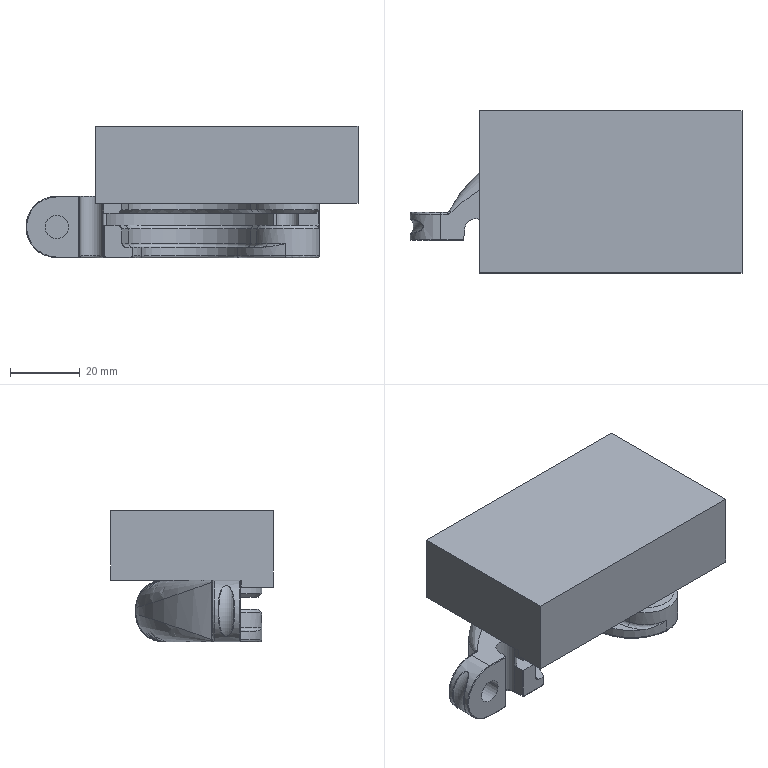NC program | NX | posted with a generic post | part box 94.951 x 46.35 x 37.6 mm
Lines 1740 to 2347 of 15115:
(ZLEVEL_PROFILE_COPY , TOOL : D6R0.5)
N3418 T23 M6
N3420 G54
N3422 G17 G0 G90 X42.811 Y-3.515 S6500 M3
N3424 G43 Z20. H23
N3426 Z-0.004
N3428 G94 G3 X42.99 Y-4.167 R2. F2500.
N3430 G2 X21.925 Y-11.674 R-11.232
N3432 G1 X20.25 Y-5.033
N3434 G3 X-10.601 Y-5.035 R15.909
N3436 G1 X-12.275 Y-11.674
N3438 G2 X-12.624 Y-12.804 R11.241
N3440 G3 X-12.738 Y-13.311 R2.
N3442 G1 X-12.683 Y-13.314 Z-0.011 F8000.
N3444 G2 X-12.57 Y-12.81 R2. F2500.
N3446 G3 X-12.223 Y-11.687 R11.295
N3448 G1 X-10.549 Y-5.048
N3450 G2 X20.199 Y-5.048 R15.855
N3452 G1 X21.873 Y-11.687
N3454 G3 X43.054 Y-4.145 R-11.292
N3456 G2 X42.876 Y-3.495 R2.
N3458 G1 X43.042 Y-3.715 Z-0.019 F8000.
N3460 G3 X43.106 Y-4.136 R1. F2500.
N3462 G2 X21.824 Y-11.699 R-11.343
N3464 G1 X20.15 Y-5.06
N3466 G3 X-10.499 Y-5.06 R15.804
N3468 G1 X-12.174 Y-11.699
N3470 G2 X-12.518 Y-12.817 R11.346
N3472 G3 X-12.631 Y-13.319 R2.
N3474 G1 X-12.58 Y-13.328 Z-0.031 F8000.
N3476 G2 X-12.467 Y-12.823 R2. F2500.
N3478 G3 X-12.126 Y-11.711 R11.395
N3480 G1 X-10.451 Y-5.072
N3482 G2 X20.101 Y-5.073 R15.755
N3484 G1 X21.776 Y-11.711
N3486 G3 X43.152 Y-4.115 R-11.393
N3488 G2 X42.976 Y-3.477 R2.
N3490 G1 X43.019 Y-3.438 Z-0.044 F8000.
N3492 G3 X43.197 Y-4.095 R2. F2500.
N3494 G2 X21.728 Y-11.723 R-11.442
N3496 G1 X20.054 Y-5.085
N3498 G3 X-10.404 Y-5.084 R15.706
N3500 G1 X-12.078 Y-11.723
N3502 G2 X-12.418 Y-12.83 R11.444
N3504 G3 X-12.53 Y-13.338 R2.
N3506 G1 X-12.481 Y-13.348 Z-0.06 F8000.
N3508 G2 X-12.369 Y-12.836 R2. F2500.
N3510 G3 X-12.032 Y-11.735 R11.492
N3512 G1 X-10.358 Y-5.096
N3514 G2 X20.008 Y-5.096 R15.658
N3516 G1 X21.682 Y-11.735
N3518 X21.709 Y-11.837
N3520 G3 X43.297 Y-4.196 R-11.49
N3522 G1 Y-4.192
N3524 X43.293 Y-4.187
N3526 X43.29 Y-4.177
N3528 X43.24 Y-4.074
N3530 G2 X43.049 Y-3.407 R2.
N3532 G1 X43.108 Y-3.414 Z-0.079 F8000.
N3534 G3 X43.284 Y-4.054 R2. F2500.
N3536 G2 X21.69 Y-11.945 R-11.537
N3538 G1 X21.636 Y-11.747
N3540 X19.962 Y-5.108
N3542 G3 X-10.312 Y-5.108 R15.611
N3544 G1 X-11.986 Y-11.747
N3546 G2 X-12.321 Y-12.842 R11.539
N3548 G3 X-12.433 Y-13.351 R2.
N3550 G1 X-12.386 Y-13.362 Z-0.099 F8000.
N3552 G2 X-12.275 Y-12.847 R2. F2500.
N3554 G3 X-11.942 Y-11.758 R11.585
N3556 G1 X-10.268 Y-5.119
N3558 G2 X19.918 Y-5.119 R15.565
N3560 G1 X21.592 Y-11.758
N3562 G3 X43.381 Y-4.156 R-11.584
N3564 G2 X43.212 Y-3.523 R2.
N3566 G1 X43.267 Y-3.532 Z-0.122 F8000.
N3568 G3 X43.38 Y-4.045 R2. F2500.
N3570 G1 X43.381 Y-4.047
N3572 X43.386 Y-4.06
N3574 X43.392 Y-4.071
N3576 X43.396 Y-4.079
N3578 Y-4.081
N3580 X43.421 Y-4.138
N3582 G2 X21.632 Y-12.066 R-11.626
N3584 G1 X21.549 Y-11.769
N3586 X19.875 Y-5.13
N3588 G3 X-10.225 Y-5.13 R15.521
N3590 G1 X-11.899 Y-11.769
N3592 G2 X-12.229 Y-12.853 R11.629
N3594 G3 X-12.34 Y-13.368 R2.
N3596 G1 X-12.296 Y-13.377 Z-0.148 F8000.
N3598 G2 X-12.185 Y-12.859 R2. F2500.
N3600 G3 X-11.857 Y-11.779 R11.673
N3602 G1 X-10.183 Y-5.141
N3604 G2 X19.832 Y-5.14 R15.477
N3606 G1 X21.507 Y-11.779
N3608 G3 X36.709 Y-19.929 R11.672
N3610 X43.424 Y-4.037 R11.672
N3612 G1 X43.405 Y-3.996
N3614 G2 X43.235 Y-3.367 R2.
N3616 G1 X43.317 Y-3.436 Z-0.175 F8000.
N3618 G3 X43.487 Y-4.072 R2. F2500.
N3620 G2 X21.466 Y-11.79 R-11.714
N3622 G1 X19.792 Y-5.151
N3624 G3 X-10.131 Y-5.11 R15.435
N3626 G1 X-10.142 Y-5.151
N3628 X-11.816 Y-11.79
N3630 G2 X-12.142 Y-12.864 R11.715
N3632 G3 X-12.252 Y-13.378 R2.
N3634 G1 X-11.831 Y-12.439 Z-0.204 F8000.
N3636 G2 X-11.776 Y-11.8 R2. F2500.
N3638 G1 X-10.103 Y-5.162
N3640 X-10.078 Y-5.065
N3642 G2 X19.752 Y-5.161 R15.395
N3644 G1 X21.426 Y-11.8
N3646 G3 X43.527 Y-4.063 R-11.755
N3648 G2 X43.357 Y-3.427 R2.
N3650 G1 X43.321 Y-3.265 Z-0.235 F8000.
N3652 G3 X43.5 Y-3.916 R2. F2500.
N3654 G2 X21.394 Y-11.825 R-11.792
N3656 G1 X21.388 Y-11.809
N3658 X19.714 Y-5.17
N3660 G3 X-9.983 Y-4.862 R15.355
N3662 X-10.065 Y-5.172 R15.355
N3664 G1 X-11.738 Y-11.809
N3666 G3 X-11.793 Y-12.449 R2.
N3668 G1 X-11.757 Y-12.458 Z-0.269 F8000.
N3670 G2 X-11.702 Y-11.818 R2. F2500.
N3672 G1 X-10.028 Y-5.181
N3674 G2 X-9.947 Y-4.872 R15.318
N3676 X19.678 Y-5.179 R15.318
N3678 G1 X21.352 Y-11.818
N3680 X21.356 Y-11.825
N3682 G3 X43.538 Y-3.909 R-11.83
N3684 G2 X43.358 Y-3.254 R2.
N3686 G1 X43.397 Y-3.252 Z-0.304 F8000.
N3688 G3 X43.575 Y-3.901 R2. F2500.
N3690 G2 X21.477 Y-12.392 R-11.866
N3692 G1 X21.317 Y-11.827
N3694 X19.643 Y-5.188
N3696 G3 X-9.994 Y-5.19 R15.282
N3698 G1 X-11.667 Y-11.827
N3700 G3 X-11.722 Y-12.467 R2.
N3702 G1 X-11.696 Y-12.496 Z-0.341 F8000.
N3704 G2 X-11.64 Y-11.855 R2. F2500.
N3706 G1 X-11.635 Y-11.835
N3708 X-9.961 Y-5.198
N3710 G2 X19.61 Y-5.196 R15.248
N3712 G1 X21.285 Y-11.835
N3714 G3 X35.515 Y-20.518 R11.909
N3716 X43.627 Y-3.929 R11.906
N3718 G2 X43.452 Y-3.284 R2.
N3720 G1 X43.502 Y-3.314 Z-0.379 F8000.
N3722 G3 X43.675 Y-3.957 R2. F2500.
N3724 G2 X21.265 Y-11.879 R-11.932
N3726 G1 X21.253 Y-11.843
N3728 X19.579 Y-5.204
N3730 G3 X-9.929 Y-5.205 R15.216
N3732 G1 X-11.603 Y-11.843
N3734 X-11.618 Y-11.899
N3736 G3 X-11.676 Y-12.54 R2.
N3738 G1 X-11.682 Y-12.657 Z-0.419 F8000.
N3740 G2 X-11.618 Y-12.018 R2. F2500.
N3742 G1 X-11.574 Y-11.85
N3744 X-9.9 Y-5.21
N3746 G2 X19.55 Y-5.212 R15.186
N3748 G1 X21.224 Y-11.851
N3750 X21.234 Y-11.889
N3752 G3 X43.669 Y-3.876 R-11.963
N3754 G2 X43.492 Y-3.225 R2.
N3756 G1 X43.582 Y-3.347 Z-0.46 F8000.
N3758 G3 X43.695 Y-3.864 R1. F2500.
N3760 G1 X43.703 Y-3.879
N3762 G2 X36.924 Y-20.193 R11.991
N3764 X21.249 Y-12.053 R11.991
N3766 G1 X21.197 Y-11.857
N3768 X19.523 Y-5.218
N3770 G3 X-9.873 Y-5.22 R15.158
N3772 G1 X-11.547 Y-11.857
N3774 G2 X-11.598 Y-12.053 R11.992
N3776 G3 X-11.664 Y-12.692 R2.
N3778 G1 X-11.672 Y-12.801 Z-0.503 F8000.
N3780 G2 X-11.601 Y-12.161 R2. F2500.
N3782 G3 X-11.522 Y-11.864 R12.018
N3784 G1 X-9.848 Y-5.226
N3786 G2 X19.498 Y-5.225 R15.132
N3788 G1 X21.172 Y-11.864
N3790 X21.227 Y-12.066
N3792 G3 X43.776 Y-3.976 R-12.016
N3794 G1 Y-3.974
N3796 X43.77 Y-3.962
N3798 X43.769 Y-3.961
N3800 X43.719 Y-3.853
N3802 G2 X43.546 Y-3.211 R2.
N3804 G1 X43.564 Y-3.195 Z-0.547 F8000.
N3806 G3 X43.741 Y-3.843 R2. F2500.
N3808 G1 X43.751 Y-3.863
N3810 X43.759 Y-3.882
N3812 G2 X21.187 Y-12.014 R-12.041
N3814 G1 X21.169 Y-11.942
N3816 X21.149 Y-11.87
N3818 X19.475 Y-5.231
N3820 G3 X-9.761 Y-4.987 R15.108
N3822 X-9.824 Y-5.229 R15.108
N3824 G1 X-11.499 Y-11.869
N3826 G2 X-11.594 Y-12.225 R12.042
N3828 G3 X-11.669 Y-12.864 R2.
N3830 G1 X-11.657 Y-12.895 Z-0.592 F8000.
N3832 G2 X-11.581 Y-12.256 R2. F2500.
N3834 G3 X-11.478 Y-11.875 R12.063
N3836 G1 X-9.804 Y-5.238
N3838 G2 X-9.725 Y-4.935 R15.087
N3840 X19.454 Y-5.236 R15.087
N3842 G1 X21.128 Y-11.875
N3844 X21.131 Y-11.884
N3846 X21.165 Y-12.014
N3848 X21.17 Y-12.032
N3850 X21.189 Y-12.104
N3852 X21.293 Y-12.461
N3854 G3 X38.641 Y-19.492 R12.062
N3856 X43.815 Y-3.954 R12.062
N3858 G1 X43.814 Y-3.95
N3860 X43.769 Y-3.852
N3862 X43.767 Y-3.849
N3864 G2 X43.563 Y-3.142 R2.
N3866 G1 X43.663 Y-3.308 Z-0.639 F8000.
N3868 G3 X43.832 Y-3.947 R2. F2500.
N3870 G2 X37.977 Y-19.852 R12.08
N3872 X22.192 Y-14.661 R12.082
N3874 X21.246 Y-12.374 R12.152
N3876 G1 X21.161 Y-12.076
N3878 X21.151 Y-12.038
N3880 X21.145 Y-12.014
N3882 X21.109 Y-11.879
N3884 X19.435 Y-5.241
N3886 G3 X-9.783 Y-5.23 R15.068
N3888 G1 X-9.786 Y-5.242
N3890 X-11.459 Y-11.879
N3892 G2 X-11.573 Y-12.299 R12.082
N3894 G3 X-11.651 Y-12.938 R2.
N3896 G1 X-11.677 Y-13.056 Z-0.686 F8000.
N3898 G2 X-11.593 Y-12.424 R2. F2500.
N3900 G3 X-11.443 Y-11.883 R12.099
N3902 G1 X-9.769 Y-5.246
N3904 X-9.752 Y-5.179
N3906 G2 X19.419 Y-5.245 R15.051
N3908 G1 X21.093 Y-11.884
N3910 X21.133 Y-12.034
N3912 G3 X43.801 Y-3.837 R-12.098
N3914 G1 X43.794 Y-3.821
N3916 X43.793 Y-3.818
N3918 G2 X43.73 Y-3.408 R2.
N3920 G1 X43.66 Y-3.227 Z-0.734 F8000.
N3922 G3 X43.834 Y-3.874 R2. F2500.
N3924 G2 X21.133 Y-12.088 R-12.113
N3926 G1 X21.079 Y-11.887
N3928 X19.405 Y-5.248
N3930 G3 X-9.755 Y-5.25 R15.036
N3932 G1 X-11.429 Y-11.887
N3934 G2 X-11.579 Y-12.428 R12.114
N3936 G3 X-11.663 Y-13.06 R2.
N3938 G1 X-11.689 Y-13.153 Z-0.782 F8000.
N3940 G2 X-11.598 Y-12.533 R2. F2500.
N3942 G3 X-11.417 Y-11.89 R12.126
N3944 G1 X-9.743 Y-5.25
N3946 X-9.697 Y-5.075
N3948 G2 X19.393 Y-5.251 R15.024
N3950 G1 X21.067 Y-11.89
N3952 X21.122 Y-12.1
N3954 X21.129 Y-12.121
N3956 G3 X36.972 Y-20.319 R12.125
N3958 X43.835 Y-3.848 R12.125
N3960 G1 X43.836 Y-3.846
N3962 X43.818 Y-3.81
N3964 G2 X43.639 Y-3.152 R2.
N3966 G1 X43.698 Y-3.253 Z-0.831 F8000.
N3968 G3 X43.869 Y-3.895 R2. F2500.
N3970 G2 X21.09 Y-12.014 R-12.135
N3972 G1 X21.058 Y-11.892
N3974 X19.384 Y-5.254
N3976 G3 X-9.72 Y-5.201 R15.014
N3978 G1 X-9.733 Y-5.252
N3980 X-11.408 Y-11.892
N3982 G2 X-11.59 Y-12.538 R12.136
N3984 G3 X-11.68 Y-13.158 R2.
N3986 G1 X-11.708 Y-13.234 Z-0.873 F8000.
N3988 G2 X-11.612 Y-12.631 R2. F2500.
N3990 G3 X-11.402 Y-11.894 R12.142
N3992 G1 X-9.727 Y-5.254
N3994 X-9.713 Y-5.2
N3996 G2 X19.377 Y-5.255 R15.008
N3998 G1 X21.052 Y-11.894
N4000 X21.084 Y-12.014
N4002 X21.122 Y-12.159
N4004 X21.136 Y-12.203
N4006 X21.175 Y-12.343
N4008 X21.189 Y-12.39
N4010 G3 X44.775 Y-11.066 R12.141
N4012 G1 X44.794 Y-10.961
N4014 X44.807 Y-10.879
N4016 X44.836 Y-10.69
N4018 X44.863 Y-10.501
N4020 G3 X43.879 Y-3.903 R12.171
N4022 G2 X43.709 Y-3.26 R2.
N4024 G1 X43.647 Y-3.122 Z-0.916 F8000.
N4026 G3 X43.834 Y-3.799 R2. F2500.
N4028 G1 X43.856 Y-3.834
N4030 X43.87 Y-3.874
N4032 X43.872 Y-3.875
N4034 X43.876 Y-3.885
N4036 Y-3.887
N4038 X43.882 Y-3.9
N4040 X43.883 Y-3.902
N4042 G2 X44.938 Y-8.043 R12.148
N4044 X44.962 Y-9.367 R12.09
N4046 X43.426 Y-14.85 R12.155
N4048 X21.729 Y-13.863 R12.145
N4050 X21.164 Y-12.32 R12.136
N4052 X21.047 Y-11.895 R15.392
N4054 G1 X19.373 Y-5.256
N4056 G3 X-9.715 Y-5.225 R15.004
N4058 G1 X-9.723 Y-5.255
N4060 X-11.397 Y-11.895
N4062 G2 X-11.611 Y-12.642 R12.146
N4064 G3 X-11.707 Y-13.242 R2.
N4066 G1 X-11.705 Y-13.245 Z-0.958 F8000.
N4068 G2 X-11.609 Y-12.643 R2. F2500.
N4070 G3 X-11.395 Y-11.896 R12.149
N4072 G1 X-9.72 Y-5.256
N4074 X-9.712 Y-5.225
N4076 G2 X19.371 Y-5.257 R15.001
N4078 G1 X21.045 Y-11.896
N4080 X21.099 Y-12.1
N4082 X21.168 Y-12.345
N4084 X21.182 Y-12.392
N4086 X21.225 Y-12.534
N4088 X21.296 Y-12.756
N4090 X21.302 Y-12.773
N4092 X21.352 Y-12.919
N4094 X21.466 Y-13.231
N4096 G3 X21.841 Y-14.114 R11.534
N4098 G1 X21.915 Y-14.269
N4100 X22.091 Y-14.614
N4102 X22.195 Y-14.805
N4104 X22.26 Y-14.921
N4106 X22.364 Y-15.1
N4108 X22.503 Y-15.33
N4110 X22.618 Y-15.513
N4112 X22.649 Y-15.56
N4114 G3 X23.002 Y-16.073 R14.847
N4116 G1 X23.028 Y-16.108
N4118 G3 X23.45 Y-16.65 R14.741
N4120 X23.662 Y-16.901 R10.518
N4122 G1 X23.753 Y-17.004
N4124 X23.789 Y-17.045
N4126 X23.894 Y-17.16
N4128 X24.026 Y-17.302
N4130 X24.123 Y-17.401
N4132 X24.169 Y-17.449
N4134 X24.344 Y-17.623
N4136 X24.457 Y-17.731
N4138 G3 X24.784 Y-18.031 R11.324
N4140 G1 X24.855 Y-18.094
N4142 G3 X25.724 Y-18.782 R11.795
N4144 G1 X25.937 Y-18.932
N4146 X25.951 Y-18.942
N4148 X26.274 Y-19.155
N4150 X26.425 Y-19.251
N4152 X26.559 Y-19.332
N4154 G3 X27.499 Y-19.843 R10.803
N4156 G1 X27.751 Y-19.963
N4158 X27.783 Y-19.977
N4160 G3 X28.153 Y-20.139 R7.631
N4162 G1 X28.263 Y-20.184
N4164 X28.593 Y-20.312
N4166 G3 X29.16 Y-20.507 R11.887
N4168 G1 X29.236 Y-20.531
N4170 X29.521 Y-20.615
N4172 X29.7 Y-20.665
N4174 G3 X30.157 Y-20.776 R11.059
N4176 G1 X30.366 Y-20.822
N4178 X30.44 Y-20.837
N4180 G3 X30.89 Y-20.918 R12.55
N4182 G1 X31.117 Y-20.953
N4184 G3 X31.662 Y-21.017 R10.961
N4186 X32.419 Y-21.066 R11.185
N4188 G1 X32.558 Y-21.07
N4190 G3 X33.099 Y-21.07 R16.498
N4192 X33.6 Y-21.049 R9.214
N4194 G1 X33.927 Y-21.023
N4196 X34.095 Y-21.006
N4198 G3 X34.883 Y-20.898 R13.803
N4200 X35.268 Y-20.825 R8.537
N4202 G1 X35.604 Y-20.751
N4204 X35.757 Y-20.715
N4206 X35.767 Y-20.712
N4208 X36.083 Y-20.628
N4210 X36.118 Y-20.618
N4212 X36.366 Y-20.546
N4214 X36.503 Y-20.503
N4216 G3 X37.022 Y-20.325 R14.958
N4218 X37.445 Y-20.161 R9.484
N4220 G1 X37.532 Y-20.125
N4222 X37.598 Y-20.096
N4224 X37.876 Y-19.974
N4226 X37.937 Y-19.946
N4228 X37.977 Y-19.926
N4230 X38.241 Y-19.799
N4232 X38.332 Y-19.754
N4234 X38.409 Y-19.713
N4236 X38.637 Y-19.593
N4238 X38.691 Y-19.563
N4240 X38.7 Y-19.559
N4242 X38.924 Y-19.432
N4244 X38.975 Y-19.402
N4246 G3 X39.5 Y-19.075 R10.738
N4248 G1 X39.639 Y-18.982
N4250 G3 X40.066 Y-18.679 R10.662
N4252 G1 X40.193 Y-18.584
N4254 X40.352 Y-18.46
N4256 X40.391 Y-18.43
N4258 G3 X41.352 Y-17.578 R12.263
N4260 G1 X41.386 Y-17.545
N4262 X41.598 Y-17.328
N4264 X41.647 Y-17.276
N4266 G3 X42.135 Y-16.73 R11.457
N4268 G1 X42.165 Y-16.693
N4270 G3 X42.427 Y-16.368 R15.526
N4272 X43.299 Y-15.079 R11.795
N4274 G1 X43.323 Y-15.039
N4276 X43.431 Y-14.85
N4278 X43.454 Y-14.808
N4280 X43.482 Y-14.757
N4282 G3 X43.705 Y-14.33 R10.538
N4284 G1 X43.78 Y-14.176
N4286 X43.841 Y-14.048
N4288 X43.887 Y-13.946
N4290 X44.023 Y-13.635
N4292 G3 X44.31 Y-12.882 R10.342
N4294 G1 X44.394 Y-12.629
N4296 X44.452 Y-12.444
N4298 X44.523 Y-12.203
N4300 X44.532 Y-12.171
N4302 X44.622 Y-11.825
N4304 X44.639 Y-11.752
N4306 X44.7 Y-11.484
N4308 X44.709 Y-11.447
N4310 X44.783 Y-11.066
N4312 X44.806 Y-10.931
N4314 X44.838 Y-10.73
N4316 G3 X44.905 Y-10.208 R9.769
N4318 G1 X44.914 Y-10.123
N4320 X44.945 Y-9.755
N4322 X44.946 Y-9.742
N4324 X44.963 Y-9.415
N4326 X44.967 Y-9.302
N4328 G3 X44.972 Y-8.773 R10.888
N4330 G1 X44.965 Y-8.49
N4332 X44.957 Y-8.303
N4334 X44.954 Y-8.231
N4336 X44.952 Y-8.208
N4338 X44.938 Y-7.997
N4340 X44.913 Y-7.722
N4342 G3 X44.815 Y-6.97 R12.459
N4344 G1 X44.802 Y-6.889
N4346 G3 X44.682 Y-6.282 R11.006
N4348 G1 X44.613 Y-5.988
N4350 X44.592 Y-5.904
N4352 G3 X44.463 Y-5.441 R11.418
N4354 G1 X44.416 Y-5.286
N4356 X44.408 Y-5.262
N4358 X44.34 Y-5.054
N4360 G3 X43.91 Y-3.954 R12.166
N4362 G1 X43.841 Y-3.806
N4364 X43.837 Y-3.797
N4366 G2 X43.71 Y-3.246 R2.
N4368 G0 Z20.
N4370 X21.099 Y-12.538
N4372 Z-1.
N4374 G3 X21.044 Y-11.896 R2.
N4376 G1 X19.37 Y-5.257
N4378 X19.367 Y-5.247
N4380 G3 X-9.641 Y-4.959 R15.
N4382 G1 X-9.671 Y-5.071
N4384 X-9.696 Y-5.163
N4386 X-9.707 Y-5.207
N4388 X-9.72 Y-5.257
N4390 X-11.394 Y-11.896
N4392 G2 X-11.456 Y-12.131 R12.15
N4394 G1 X-11.472 Y-12.191
N4396 G2 X-11.608 Y-12.643 R12.15
N4398 G3 X-11.704 Y-13.245 R2.
N4400 G0 Z20.
N4402 M5
(PLANAR_MILL_1 , TOOL : T_CUTTER_1)
N4404 T06 M6
N4406 G54
N4408 G17 G0 G90 X51.908 Y-5.698 S2000 M3
N4410 G43 Z20. H6
N4412 Z-5.1
N4414 G94 G1 Z-8.1 F180.
N4416 G3 X49.171 Y-8.56 R2.8
N4418 G2 X41.773 Y-16.125 R7.4 F300.
N4420 G1 X28.907
N4422 G2 X21.732 Y-10.534 R7.4
N4424 G1 X20.339 Y-5.013
N4426 G3 X-10.689 Y-5.013 R16.
N4428 G1 X-12.092 Y-10.575
N4430 G3 X-4.841 Y-22.717 R10.
N4432 G1 Z-1.1
N4434 G0 Z20.
(PLANAR_MILL_1_COPY , TOOL : T_CUTTER_1)
N4436 X51.908 Y-5.699
N4438 Z-4.85
N4440 G1 Z-7.85 F180.
N4442 G41 X51.708 Y-5.702 D6
N4444 G3 X48.971 Y-8.564 R2.8
N4446 G2 X41.773 Y-15.925 R7.2 F300.
N4448 G1 X28.907
N4450 G2 X21.926 Y-10.486 R7.2
N4452 G1 X20.533 Y-4.964
N4454 G3 X-10.883 Y-4.964 R16.2
N4456 G1 X-12.286 Y-10.527
N4458 G3 X-5.035 Y-22.668 R10.
N4460 G40
N4462 G1 X-4.841 Y-22.716
N4464 Z-0.85
N4466 G0 Z20.
(PLANAR_MILL_1_COPY_COPY , TOOL : T_CUTTER_1)
N4468 X51.908 Y-5.699
N4470 Z-5.35
N4472 G1 Z-8.35 F180.
N4474 G41 X51.708 Y-5.702
N4476 G3 X48.971 Y-8.564 R2.8
N4478 G2 X41.773 Y-15.925 R7.2 F300.
N4480 G1 X28.907
N4482 G2 X21.926 Y-10.486 R7.2
N4484 G1 X20.533 Y-4.964
N4486 G3 X-10.883 Y-4.964 R16.2
N4488 G1 X-12.286 Y-10.527
N4490 G3 X-5.035 Y-22.668 R10.
N4492 G40
N4494 G1 X-4.841 Y-22.716
N4496 Z-1.35
N4498 G0 Z20.
N4500 M5
(PLANAR_MILL_2 , TOOL : 倒角3.)
N4502 T12 M6
N4504 G54
N4506 G17 G0 G90 X35.827 Y-11.444 S5500 M3
N4508 G43 Z20. H12
N4510 Z2.2
N4512 G94 G1 Z-0.8 F1000.
N4514 X36.976 Y-12.408
N4516 X37.351 Y-11.962
N4518 G3 X36.601 Y-12.855 R-5.45
N4520 G1 X36.976 Y-12.408
N4522 X35.827 Y-11.444
N4524 Z2.2
N4526 G0 Z20.
N4528 X-12.762 Y-12.725
N4530 Z2.2
N4532 G1 Z-0.8
N4534 X-15.062
N4536 X-19.7
N4538 G2 X-20.497 Y-11.995 R0.8
N4540 G1 X-20.784 Y-8.716
N4542 G3 X-25.566 Y-8.716 R2.4
N4544 G1 X-25.835 Y-11.795
N4546 X-26.036 Y-14.086
N4548 Z2.2
N4550 G0 Z20.
(PLANAR_MILL_2_COPY , TOOL : 倒角3.)
N4552 X31.325 Y-8.925
N4554 Z1.2
N4556 G1 Z-1.8
N4558 X29.825
N4560 G3 X32.825 Y-11.925 R3.
N4562 X29.825 Y-8.925 R-3.
N4564 G1 X31.325
N4566 Z1.2
N4568 G0 Z20.
(PLANAR_MILL_2_COPY_COPY , TOOL : 倒角3.)
N4570 X25.644 Y-19.534
N4572 Z-12.6
N4574 G1 Z-15.6
N4576 G3 X24.965 Y-16.788 R2.
N4578 G2 X17.559 Y-6.309 R16.
N4580 G3 X-7.909 Y-6.309 R13.
N4582 G2 X-10.588 Y-12.425 R16.
N4584 G3 X-10.131 Y-15.216 R2.
N4586 G1 Z-12.6
N4588 G0 Z20.
N4590 M5